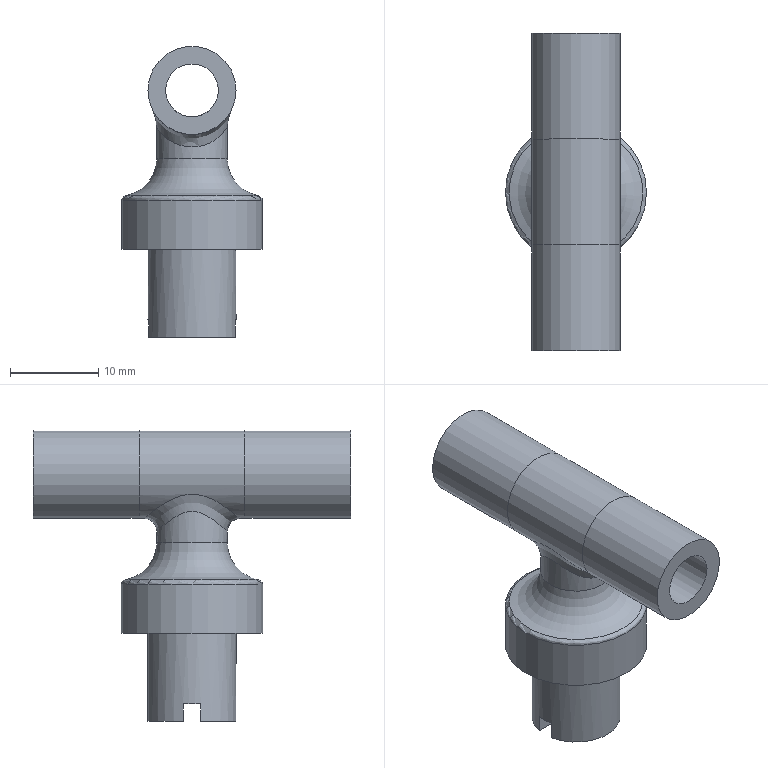Part | STEP file | 1-55.2 | 1 solid | 22 faces | box 16 x 36 x 33 mm | volume 3784 mm3 | plane 11 | cylinder 8 | torus 2 | spline 1 | commonest cylinder face diameters 10 x4 5 x1 6 x1 8 x1 16 x1